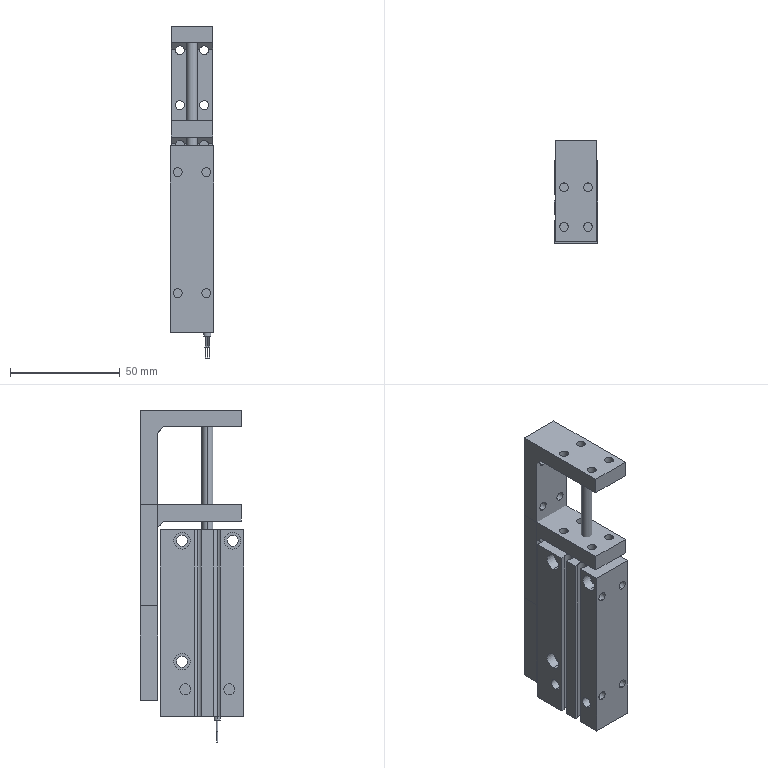Part | NX | 6 solids | 303 faces | box 20 x 47 x 151 mm | volume 111362 mm3 | cylinder 172 | plane 117 | torus 6 | cone 4 | spline 4 | commonest cylinder face diameters 4 x82 5 x26 0.5 x12 0.75 x12 7.5 x12 2.05 x8